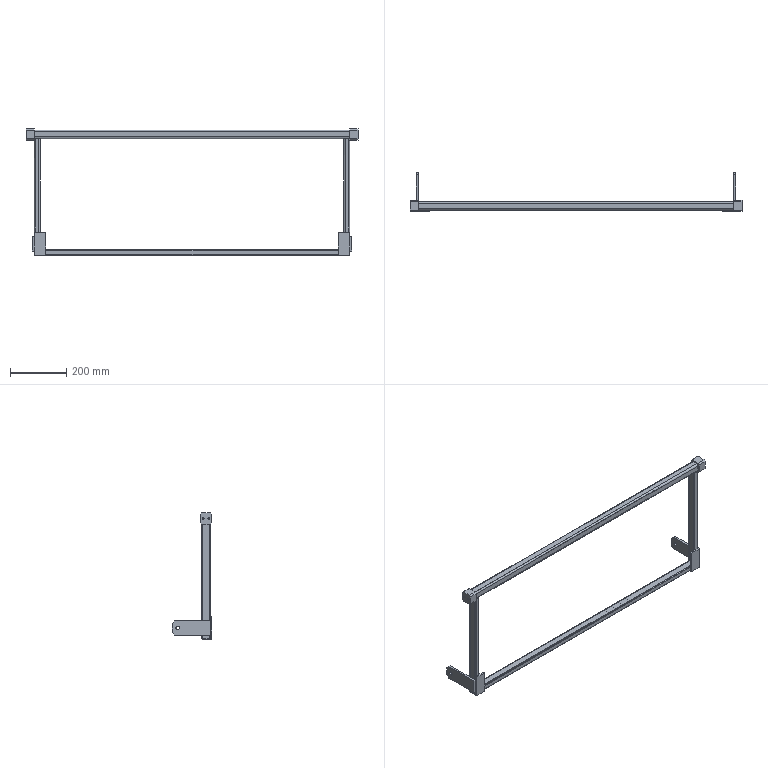Part | SolidWorks | features ICE 5, 3DProfileFeature 4, HoleWzd 2, WeldMemberFeat 2, MirrorPattern 1, WeldmentFeature 1 | 7 solids | 156 faces | box 1176 x 141 x 448 mm | volume 897407 mm3 | plane 92 | cylinder 52 | cone 12 | commonest cylinder face diameters 4 x12 8 x12 5 x8 6.8 x8 6 x4 12 x4